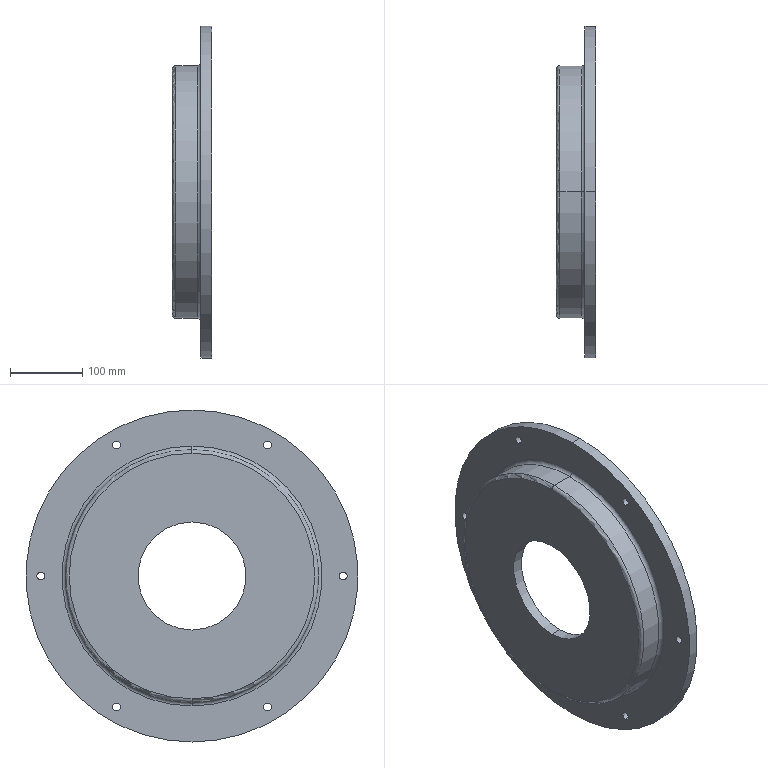Part | SolidWorks | features Cut 1, Revolution 1 | 1 solid | 32 faces | box 54.8 x 461 x 461 mm | volume 2855101 mm3 | cylinder 20 | torus 8 | plane 4 | commonest cylinder face diameters 11 x12 150 x2 321 x2 351 x2 461 x2
STEP:
#1=CARTESIAN_POINT('',(-352.644,210.,5.5));
#2=VERTEX_POINT('',#1);
#3=CARTESIAN_POINT('',(-352.644,210.,-5.5));
#4=VERTEX_POINT('',#3);
#5=CARTESIAN_POINT('',(-352.644,210.,0.));
#6=DIRECTION('',(1.,0.,0.));
#7=DIRECTION('',(0.,0.,-1.));
#8=AXIS2_PLACEMENT_3D('',#5,#6,#7);
#9=CIRCLE('',#8,5.5);
#10=EDGE_CURVE('',#2,#4,#9,.T.);
#11=ORIENTED_EDGE('',*,*,#10,.T.);
#12=CARTESIAN_POINT('',(-367.644,210.,-5.5));
#13=VERTEX_POINT('',#12);
#14=CARTESIAN_POINT('',(-282.644,210.,-5.5));
#15=DIRECTION('',(-1.,0.,0.));
#16=VECTOR('',#15,1000.);
#17=LINE('',#14,#16);
#18=EDGE_CURVE('',#4,#13,#17,.T.);
#19=ORIENTED_EDGE('',*,*,#18,.T.);
#20=CARTESIAN_POINT('',(-367.644,210.,5.5));
#21=VERTEX_POINT('',#20);
#22=CARTESIAN_POINT('',(-367.644,210.,0.));
#23=DIRECTION('',(-1.,0.,0.));
#24=DIRECTION('',(0.,0.,1.));
#25=AXIS2_PLACEMENT_3D('',#22,#23,#24);
#26=CIRCLE('',#25,5.5);
#27=EDGE_CURVE('',#13,#21,#26,.T.);
#28=ORIENTED_EDGE('',*,*,#27,.T.);
#29=CARTESIAN_POINT('',(-282.644,210.,5.5));
#30=DIRECTION('',(-1.,0.,0.));
#31=VECTOR('',#30,1000.);
#32=LINE('',#29,#31);
#33=EDGE_CURVE('',#2,#21,#32,.T.);
#34=ORIENTED_EDGE('',*,*,#33,.F.);
#35=EDGE_LOOP('',(#11,#19,#28,#34));
#36=FACE_OUTER_BOUND('',#35,.T.);
#37=CARTESIAN_POINT('',(-282.644,210.,0.));
#38=DIRECTION('',(-1.,0.,0.));
#39=DIRECTION('',(0.,0.,1.));
#40=AXIS2_PLACEMENT_3D('',#37,#38,#39);
#41=CYLINDRICAL_SURFACE('',#40,5.5);
#42=ADVANCED_FACE('',(#36),#41,.F.);
#43=CARTESIAN_POINT('',(-352.644,105.,-176.365));
#44=VERTEX_POINT('',#43);
#45=CARTESIAN_POINT('',(-352.644,105.,-187.365));
#46=VERTEX_POINT('',#45);
#47=CARTESIAN_POINT('',(-352.644,105.,-181.865));
#48=DIRECTION('',(1.,0.,0.));
#49=DIRECTION('',(0.,0.,-1.));
#50=AXIS2_PLACEMENT_3D('',#47,#48,#49);
#51=CIRCLE('',#50,5.5);
#52=EDGE_CURVE('',#44,#46,#51,.T.);
#53=ORIENTED_EDGE('',*,*,#52,.T.);
#54=CARTESIAN_POINT('',(-367.644,105.,-187.365));
#55=VERTEX_POINT('',#54);
#56=CARTESIAN_POINT('',(-282.644,105.,-187.365));
#57=DIRECTION('',(-1.,0.,0.));
#58=VECTOR('',#57,1000.);
#59=LINE('',#56,#58);
#60=EDGE_CURVE('',#46,#55,#59,.T.);
#61=ORIENTED_EDGE('',*,*,#60,.T.);
#62=CARTESIAN_POINT('',(-367.644,105.,-176.365));
#63=VERTEX_POINT('',#62);
#64=CARTESIAN_POINT('',(-367.644,105.,-181.865));
#65=DIRECTION('',(-1.,0.,0.));
#66=DIRECTION('',(0.,0.,1.));
#67=AXIS2_PLACEMENT_3D('',#64,#65,#66);
#68=CIRCLE('',#67,5.5);
#69=EDGE_CURVE('',#55,#63,#68,.T.);
#70=ORIENTED_EDGE('',*,*,#69,.T.);
#71=CARTESIAN_POINT('',(-282.644,105.,-176.365));
#72=DIRECTION('',(-1.,0.,0.));
#73=VECTOR('',#72,1000.);
#74=LINE('',#71,#73);
#75=EDGE_CURVE('',#44,#63,#74,.T.);
#76=ORIENTED_EDGE('',*,*,#75,.F.);
#77=EDGE_LOOP('',(#53,#61,#70,#76));
#78=FACE_OUTER_BOUND('',#77,.T.);
#79=CARTESIAN_POINT('',(-282.644,105.,-181.865));
#80=DIRECTION('',(-1.,0.,0.));
#81=DIRECTION('',(0.,0.,1.));
#82=AXIS2_PLACEMENT_3D('',#79,#80,#81);
#83=CYLINDRICAL_SURFACE('',#82,5.5);
#84=ADVANCED_FACE('',(#78),#83,.F.);
#85=CARTESIAN_POINT('',(-352.644,-105.,-176.365));
#86=VERTEX_POINT('',#85);
#87=CARTESIAN_POINT('',(-352.644,-105.,-187.365));
#88=VERTEX_POINT('',#87);
#89=CARTESIAN_POINT('',(-352.644,-105.,-181.865));
#90=DIRECTION('',(1.,0.,0.));
#91=DIRECTION('',(0.,0.,-1.));
#92=AXIS2_PLACEMENT_3D('',#89,#90,#91);
#93=CIRCLE('',#92,5.5);
#94=EDGE_CURVE('',#86,#88,#93,.T.);
#95=ORIENTED_EDGE('',*,*,#94,.T.);
#96=CARTESIAN_POINT('',(-367.644,-105.,-187.365));
#97=VERTEX_POINT('',#96);
#98=CARTESIAN_POINT('',(-282.644,-105.,-187.365));
#99=DIRECTION('',(-1.,0.,0.));
#100=VECTOR('',#99,1000.);
#101=LINE('',#98,#100);
#102=EDGE_CURVE('',#88,#97,#101,.T.);
#103=ORIENTED_EDGE('',*,*,#102,.T.);
#104=CARTESIAN_POINT('',(-367.644,-105.,-176.365));
#105=VERTEX_POINT('',#104);
#106=CARTESIAN_POINT('',(-367.644,-105.,-181.865));
#107=DIRECTION('',(-1.,0.,0.));
#108=DIRECTION('',(0.,0.,1.));
#109=AXIS2_PLACEMENT_3D('',#106,#107,#108);
#110=CIRCLE('',#109,5.5);
#111=EDGE_CURVE('',#97,#105,#110,.T.);
#112=ORIENTED_EDGE('',*,*,#111,.T.);
#113=CARTESIAN_POINT('',(-282.644,-105.,-176.365));
#114=DIRECTION('',(-1.,0.,0.));
#115=VECTOR('',#114,1000.);
#116=LINE('',#113,#115);
#117=EDGE_CURVE('',#86,#105,#116,.T.);
#118=ORIENTED_EDGE('',*,*,#117,.F.);
#119=EDGE_LOOP('',(#95,#103,#112,#118));
#120=FACE_OUTER_BOUND('',#119,.T.);
#121=CARTESIAN_POINT('',(-282.644,-105.,-181.865));
#122=DIRECTION('',(-1.,0.,0.));
#123=DIRECTION('',(0.,0.,1.));
#124=AXIS2_PLACEMENT_3D('',#121,#122,#123);
#125=CYLINDRICAL_SURFACE('',#124,5.5);
#126=ADVANCED_FACE('',(#120),#125,.F.);
#127=CARTESIAN_POINT('',(-352.644,-210.,5.5));
#128=VERTEX_POINT('',#127);
#129=CARTESIAN_POINT('',(-352.644,-210.,-5.5));
#130=VERTEX_POINT('',#129);
#131=CARTESIAN_POINT('',(-352.644,-210.,0.));
#132=DIRECTION('',(1.,0.,0.));
#133=DIRECTION('',(0.,0.,-1.));
#134=AXIS2_PLACEMENT_3D('',#131,#132,#133);
#135=CIRCLE('',#134,5.5);
#136=EDGE_CURVE('',#128,#130,#135,.T.);
#137=ORIENTED_EDGE('',*,*,#136,.T.);
#138=CARTESIAN_POINT('',(-367.644,-210.,-5.5));
#139=VERTEX_POINT('',#138);
#140=CARTESIAN_POINT('',(-282.644,-210.,-5.5));
#141=DIRECTION('',(-1.,0.,0.));
#142=VECTOR('',#141,1000.);
#143=LINE('',#140,#142);
#144=EDGE_CURVE('',#130,#139,#143,.T.);
#145=ORIENTED_EDGE('',*,*,#144,.T.);
#146=CARTESIAN_POINT('',(-367.644,-210.,5.5));
#147=VERTEX_POINT('',#146);
#148=CARTESIAN_POINT('',(-367.644,-210.,0.));
#149=DIRECTION('',(-1.,0.,0.));
#150=DIRECTION('',(0.,0.,1.));
#151=AXIS2_PLACEMENT_3D('',#148,#149,#150);
#152=CIRCLE('',#151,5.5);
#153=EDGE_CURVE('',#139,#147,#152,.T.);
#154=ORIENTED_EDGE('',*,*,#153,.T.);
#155=CARTESIAN_POINT('',(-282.644,-210.,5.5));
#156=DIRECTION('',(-1.,0.,0.));
#157=VECTOR('',#156,1000.);
#158=LINE('',#155,#157);
#159=EDGE_CURVE('',#128,#147,#158,.T.);
#160=ORIENTED_EDGE('',*,*,#159,.F.);
#161=EDGE_LOOP('',(#137,#145,#154,#160));
#162=FACE_OUTER_BOUND('',#161,.T.);
#163=CARTESIAN_POINT('',(-282.644,-210.,0.));
#164=DIRECTION('',(-1.,0.,0.));
#165=DIRECTION('',(0.,0.,1.));
#166=AXIS2_PLACEMENT_3D('',#163,#164,#165);
#167=CYLINDRICAL_SURFACE('',#166,5.5);
#168=ADVANCED_FACE('',(#162),#167,.F.);
#169=CARTESIAN_POINT('',(-352.644,-105.,187.365));
#170=VERTEX_POINT('',#169);
#171=CARTESIAN_POINT('',(-352.644,-105.,176.365));
#172=VERTEX_POINT('',#171);
#173=CARTESIAN_POINT('',(-352.644,-105.,181.865));
#174=DIRECTION('',(1.,0.,0.));
#175=DIRECTION('',(0.,0.,-1.));
#176=AXIS2_PLACEMENT_3D('',#173,#174,#175);
#177=CIRCLE('',#176,5.5);
#178=EDGE_CURVE('',#170,#172,#177,.T.);
#179=ORIENTED_EDGE('',*,*,#178,.T.);
#180=CARTESIAN_POINT('',(-367.644,-105.,176.365));
#181=VERTEX_POINT('',#180);
#182=CARTESIAN_POINT('',(-282.644,-105.,176.365));
#183=DIRECTION('',(-1.,0.,0.));
#184=VECTOR('',#183,1000.);
#185=LINE('',#182,#184);
#186=EDGE_CURVE('',#172,#181,#185,.T.);
#187=ORIENTED_EDGE('',*,*,#186,.T.);
#188=CARTESIAN_POINT('',(-367.644,-105.,187.365));
#189=VERTEX_POINT('',#188);
#190=CARTESIAN_POINT('',(-367.644,-105.,181.865));
#191=DIRECTION('',(-1.,0.,0.));
#192=DIRECTION('',(0.,0.,1.));
#193=AXIS2_PLACEMENT_3D('',#190,#191,#192);
#194=CIRCLE('',#193,5.5);
#195=EDGE_CURVE('',#181,#189,#194,.T.);
#196=ORIENTED_EDGE('',*,*,#195,.T.);
#197=CARTESIAN_POINT('',(-282.644,-105.,187.365));
#198=DIRECTION('',(-1.,0.,0.));
#199=VECTOR('',#198,1000.);
#200=LINE('',#197,#199);
#201=EDGE_CURVE('',#170,#189,#200,.T.);
#202=ORIENTED_EDGE('',*,*,#201,.F.);
#203=EDGE_LOOP('',(#179,#187,#196,#202));
#204=FACE_OUTER_BOUND('',#203,.T.);
#205=CARTESIAN_POINT('',(-282.644,-105.,181.865));
#206=DIRECTION('',(-1.,0.,0.));
#207=DIRECTION('',(0.,0.,1.));
#208=AXIS2_PLACEMENT_3D('',#205,#206,#207);
#209=CYLINDRICAL_SURFACE('',#208,5.5);
#210=ADVANCED_FACE('',(#204),#209,.F.);
#211=CARTESIAN_POINT('',(-352.644,105.,187.365));
#212=VERTEX_POINT('',#211);
#213=CARTESIAN_POINT('',(-352.644,105.,176.365));
#214=VERTEX_POINT('',#213);
#215=CARTESIAN_POINT('',(-352.644,105.,181.865));
#216=DIRECTION('',(1.,0.,0.));
#217=DIRECTION('',(0.,0.,-1.));
#218=AXIS2_PLACEMENT_3D('',#215,#216,#217);
#219=CIRCLE('',#218,5.5);
#220=EDGE_CURVE('',#212,#214,#219,.T.);
#221=ORIENTED_EDGE('',*,*,#220,.T.);
#222=CARTESIAN_POINT('',(-367.644,105.,176.365));
#223=VERTEX_POINT('',#222);
#224=CARTESIAN_POINT('',(-282.644,105.,176.365));
#225=DIRECTION('',(-1.,0.,0.));
#226=VECTOR('',#225,1000.);
#227=LINE('',#224,#226);
#228=EDGE_CURVE('',#214,#223,#227,.T.);
#229=ORIENTED_EDGE('',*,*,#228,.T.);
#230=CARTESIAN_POINT('',(-367.644,105.,187.365));
#231=VERTEX_POINT('',#230);
#232=CARTESIAN_POINT('',(-367.644,105.,181.865));
#233=DIRECTION('',(-1.,0.,0.));
#234=DIRECTION('',(0.,0.,1.));
#235=AXIS2_PLACEMENT_3D('',#232,#233,#234);
#236=CIRCLE('',#235,5.5);
#237=EDGE_CURVE('',#223,#231,#236,.T.);
#238=ORIENTED_EDGE('',*,*,#237,.T.);
#239=CARTESIAN_POINT('',(-282.644,105.,187.365));
#240=DIRECTION('',(-1.,0.,0.));
#241=VECTOR('',#240,1000.);
#242=LINE('',#239,#241);
#243=EDGE_CURVE('',#212,#231,#242,.T.);
#244=ORIENTED_EDGE('',*,*,#243,.F.);
#245=EDGE_LOOP('',(#221,#229,#238,#244));
#246=FACE_OUTER_BOUND('',#245,.T.);
#247=CARTESIAN_POINT('',(-282.644,105.,181.865));
#248=DIRECTION('',(-1.,0.,0.));
#249=DIRECTION('',(0.,0.,1.));
#250=AXIS2_PLACEMENT_3D('',#247,#248,#249);
#251=CYLINDRICAL_SURFACE('',#250,5.5);
#252=ADVANCED_FACE('',(#246),#251,.F.);
#253=CARTESIAN_POINT('',(-391.444,0.,160.5));
#254=VERTEX_POINT('',#253);
#255=CARTESIAN_POINT('',(-391.444,0.,-160.5));
#256=VERTEX_POINT('',#255);
#257=CARTESIAN_POINT('',(-391.444,0.,0.));
#258=DIRECTION('',(1.,0.,0.));
#259=DIRECTION('',(0.,0.,-1.));
#260=AXIS2_PLACEMENT_3D('',#257,#258,#259);
#261=CIRCLE('',#260,160.5);
#262=EDGE_CURVE('',#254,#256,#261,.T.);
#263=ORIENTED_EDGE('',*,*,#262,.F.);
#264=CARTESIAN_POINT('',(-357.644,0.,160.5));
#265=VERTEX_POINT('',#264);
#266=CARTESIAN_POINT('',(0.,0.,160.5));
#267=DIRECTION('',(1.,0.,0.));
#268=VECTOR('',#267,1000.);
#269=LINE('',#266,#268);
#270=EDGE_CURVE('',#254,#265,#269,.T.);
#271=ORIENTED_EDGE('',*,*,#270,.T.);
#272=CARTESIAN_POINT('',(-357.644,0.,-160.5));
#273=VERTEX_POINT('',#272);
#274=CARTESIAN_POINT('',(-357.644,0.,0.));
#275=DIRECTION('',(1.,0.,0.));
#276=DIRECTION('',(0.,0.,-1.));
#277=AXIS2_PLACEMENT_3D('',#274,#275,#276);
#278=CIRCLE('',#277,160.5);
#279=EDGE_CURVE('',#265,#273,#278,.T.);
#280=ORIENTED_EDGE('',*,*,#279,.T.);
#281=CARTESIAN_POINT('',(0.,0.,-160.5));
#282=DIRECTION('',(1.,0.,0.));
#283=VECTOR('',#282,1000.);
#284=LINE('',#281,#283);
#285=EDGE_CURVE('',#256,#273,#284,.T.);
#286=ORIENTED_EDGE('',*,*,#285,.F.);
#287=EDGE_LOOP('',(#263,#271,#280,#286));
#288=FACE_OUTER_BOUND('',#287,.T.);
#289=CARTESIAN_POINT('',(0.,0.,0.));
#290=DIRECTION('',(1.,0.,0.));
#291=DIRECTION('',(0.,0.,-1.));
#292=AXIS2_PLACEMENT_3D('',#289,#290,#291);
#293=CYLINDRICAL_SURFACE('',#292,160.5);
#294=ADVANCED_FACE('',(#288),#293,.F.);
#295=CARTESIAN_POINT('',(-392.444,0.,159.5));
#296=VERTEX_POINT('',#295);
#297=CARTESIAN_POINT('',(-392.444,0.,-159.5));
#298=VERTEX_POINT('',#297);
#299=CARTESIAN_POINT('',(-392.444,0.,0.));
#300=DIRECTION('',(1.,0.,0.));
#301=DIRECTION('',(0.,0.,-1.));
#302=AXIS2_PLACEMENT_3D('',#299,#300,#301);
#303=CIRCLE('',#302,159.5);
#304=EDGE_CURVE('',#296,#298,#303,.T.);
#305=ORIENTED_EDGE('',*,*,#304,.F.);
#306=CARTESIAN_POINT('',(-391.444,0.,159.5));
#307=DIRECTION('',(0.,1.,0.));
#308=DIRECTION('',(0.,0.,1.));
#309=AXIS2_PLACEMENT_3D('',#306,#307,#308);
#310=CIRCLE('',#309,1.);
#311=EDGE_CURVE('',#296,#254,#310,.T.);
#312=ORIENTED_EDGE('',*,*,#311,.T.);
#313=ORIENTED_EDGE('',*,*,#262,.T.);
#314=CARTESIAN_POINT('',(-391.444,0.,-159.5));
#315=DIRECTION('',(0.,-1.,0.));
#316=DIRECTION('',(0.,0.,-1.));
#317=AXIS2_PLACEMENT_3D('',#314,#315,#316);
#318=CIRCLE('',#317,1.);
#319=EDGE_CURVE('',#298,#256,#318,.T.);
#320=ORIENTED_EDGE('',*,*,#319,.F.);
#321=EDGE_LOOP('',(#305,#312,#313,#320));
#322=FACE_OUTER_BOUND('',#321,.T.);
#323=CARTESIAN_POINT('',(-391.444,0.,0.));
#324=DIRECTION('',(1.,0.,0.));
#325=DIRECTION('',(0.,0.,-1.));
#326=AXIS2_PLACEMENT_3D('',#323,#324,#325);
#327=TOROIDAL_SURFACE('',#326,159.5,1.);
#328=ADVANCED_FACE('',(#322),#327,.F.);
#329=CARTESIAN_POINT('',(-407.444,0.,75.));
#330=VERTEX_POINT('',#329);
#331=CARTESIAN_POINT('',(-407.444,0.,-75.));
#332=VERTEX_POINT('',#331);
#333=CARTESIAN_POINT('',(-407.444,0.,0.));
#334=DIRECTION('',(1.,0.,0.));
#335=DIRECTION('',(0.,0.,-1.));
#336=AXIS2_PLACEMENT_3D('',#333,#334,#335);
#337=CIRCLE('',#336,75.);
#338=EDGE_CURVE('',#330,#332,#337,.T.);
#339=ORIENTED_EDGE('',*,*,#338,.F.);
#340=CARTESIAN_POINT('',(-392.444,0.,75.));
#341=VERTEX_POINT('',#340);
#342=CARTESIAN_POINT('',(0.,0.,75.));
#343=DIRECTION('',(1.,0.,0.));
#344=VECTOR('',#343,1000.);
#345=LINE('',#342,#344);
#346=EDGE_CURVE('',#330,#341,#345,.T.);
#347=ORIENTED_EDGE('',*,*,#346,.T.);
#348=CARTESIAN_POINT('',(-392.444,0.,-75.));
#349=VERTEX_POINT('',#348);
#350=CARTESIAN_POINT('',(-392.444,0.,0.));
#351=DIRECTION('',(1.,0.,0.));
#352=DIRECTION('',(0.,0.,-1.));
#353=AXIS2_PLACEMENT_3D('',#350,#351,#352);
#354=CIRCLE('',#353,75.);
#355=EDGE_CURVE('',#341,#349,#354,.T.);
#356=ORIENTED_EDGE('',*,*,#355,.T.);
#357=CARTESIAN_POINT('',(0.,0.,-75.));
#358=DIRECTION('',(1.,0.,0.));
#359=VECTOR('',#358,1000.);
#360=LINE('',#357,#359);
#361=EDGE_CURVE('',#332,#349,#360,.T.);
#362=ORIENTED_EDGE('',*,*,#361,.F.);
#363=EDGE_LOOP('',(#339,#347,#356,#362));
#364=FACE_OUTER_BOUND('',#363,.T.);
#365=CARTESIAN_POINT('',(0.,0.,0.));
#366=DIRECTION('',(1.,0.,0.));
#367=DIRECTION('',(0.,0.,-1.));
#368=AXIS2_PLACEMENT_3D('',#365,#366,#367);
#369=CYLINDRICAL_SURFACE('',#368,75.);
#370=ADVANCED_FACE('',(#364),#369,.F.);
#371=CARTESIAN_POINT('',(-407.444,0.,-170.5));
#372=VERTEX_POINT('',#371);
#373=CARTESIAN_POINT('',(-407.444,0.,170.5));
#374=VERTEX_POINT('',#373);
#375=CARTESIAN_POINT('',(-407.444,0.,0.));
#376=DIRECTION('',(1.,0.,0.));
#377=DIRECTION('',(0.,0.,-1.));
#378=AXIS2_PLACEMENT_3D('',#375,#376,#377);
#379=CIRCLE('',#378,170.5);
#380=EDGE_CURVE('',#372,#374,#379,.T.);
#381=ORIENTED_EDGE('',*,*,#380,.T.);
#382=CARTESIAN_POINT('',(-402.444,0.,175.5));
#383=VERTEX_POINT('',#382);
#384=CARTESIAN_POINT('',(-402.444,0.,170.5));
#385=DIRECTION('',(0.,1.,0.));
#386=DIRECTION('',(0.,0.,1.));
#387=AXIS2_PLACEMENT_3D('',#384,#385,#386);
#388=CIRCLE('',#387,5.);
#389=EDGE_CURVE('',#374,#383,#388,.T.);
#390=ORIENTED_EDGE('',*,*,#389,.T.);
#391=CARTESIAN_POINT('',(-402.444,0.,-175.5));
#392=VERTEX_POINT('',#391);
#393=CARTESIAN_POINT('',(-402.444,0.,0.));
#394=DIRECTION('',(1.,0.,0.));
#395=DIRECTION('',(0.,0.,-1.));
#396=AXIS2_PLACEMENT_3D('',#393,#394,#395);
#397=CIRCLE('',#396,175.5);
#398=EDGE_CURVE('',#392,#383,#397,.T.);
#399=ORIENTED_EDGE('',*,*,#398,.F.);
#400=CARTESIAN_POINT('',(-402.444,0.,-170.5));
#401=DIRECTION('',(0.,-1.,0.));
#402=DIRECTION('',(0.,0.,-1.));
#403=AXIS2_PLACEMENT_3D('',#400,#401,#402);
#404=CIRCLE('',#403,5.);
#405=EDGE_CURVE('',#372,#392,#404,.T.);
#406=ORIENTED_EDGE('',*,*,#405,.F.);
#407=EDGE_LOOP('',(#381,#390,#399,#406));
#408=FACE_OUTER_BOUND('',#407,.T.);
#409=CARTESIAN_POINT('',(-402.444,0.,0.));
#410=DIRECTION('',(1.,0.,0.));
#411=DIRECTION('',(0.,0.,-1.));
#412=AXIS2_PLACEMENT_3D('',#409,#410,#411);
#413=TOROIDAL_SURFACE('',#412,170.5,5.);
#414=ADVANCED_FACE('',(#408),#413,.T.);
#415=ORIENTED_EDGE('',*,*,#398,.T.);
#416=CARTESIAN_POINT('',(-372.644,0.,175.5));
#417=VERTEX_POINT('',#416);
#418=CARTESIAN_POINT('',(0.,0.,175.5));
#419=DIRECTION('',(1.,0.,0.));
#420=VECTOR('',#419,1000.);
#421=LINE('',#418,#420);
#422=EDGE_CURVE('',#383,#417,#421,.T.);
#423=ORIENTED_EDGE('',*,*,#422,.T.);
#424=CARTESIAN_POINT('',(-372.644,0.,-175.5));
#425=VERTEX_POINT('',#424);
#426=CARTESIAN_POINT('',(-372.644,0.,0.));
#427=DIRECTION('',(1.,0.,0.));
#428=DIRECTION('',(0.,0.,-1.));
#429=AXIS2_PLACEMENT_3D('',#426,#427,#428);
#430=CIRCLE('',#429,175.5);
#431=EDGE_CURVE('',#425,#417,#430,.T.);
#432=ORIENTED_EDGE('',*,*,#431,.F.);
#433=CARTESIAN_POINT('',(0.,0.,-175.5));
#434=DIRECTION('',(1.,0.,0.));
#435=VECTOR('',#434,1000.);
#436=LINE('',#433,#435);
#437=EDGE_CURVE('',#392,#425,#436,.T.);
#438=ORIENTED_EDGE('',*,*,#437,.F.);
#439=EDGE_LOOP('',(#415,#423,#432,#438));
#440=FACE_OUTER_BOUND('',#439,.T.);
#441=CARTESIAN_POINT('',(0.,0.,0.));
#442=DIRECTION('',(1.,0.,0.));
#443=DIRECTION('',(0.,0.,-1.));
#444=AXIS2_PLACEMENT_3D('',#441,#442,#443);
#445=CYLINDRICAL_SURFACE('',#444,175.5);
#446=ADVANCED_FACE('',(#440),#445,.T.);
#447=CARTESIAN_POINT('',(-367.644,0.,180.5));
#448=VERTEX_POINT('',#447);
#449=CARTESIAN_POINT('',(-367.644,0.,-180.5));
#450=VERTEX_POINT('',#449);
#451=CARTESIAN_POINT('',(-367.644,0.,0.));
#452=DIRECTION('',(1.,0.,0.));
#453=DIRECTION('',(0.,0.,-1.));
#454=AXIS2_PLACEMENT_3D('',#451,#452,#453);
#455=CIRCLE('',#454,180.5);
#456=EDGE_CURVE('',#448,#450,#455,.T.);
#457=ORIENTED_EDGE('',*,*,#456,.F.);
#458=CARTESIAN_POINT('',(-372.644,0.,180.5));
#459=DIRECTION('',(0.,1.,0.));
#460=DIRECTION('',(0.,0.,1.));
#461=AXIS2_PLACEMENT_3D('',#458,#459,#460);
#462=CIRCLE('',#461,5.);
#463=EDGE_CURVE('',#448,#417,#462,.T.);
#464=ORIENTED_EDGE('',*,*,#463,.T.);
#465=CARTESIAN_POINT('',(-372.644,0.,0.));
#466=DIRECTION('',(1.,0.,0.));
#467=DIRECTION('',(0.,0.,-1.));
#468=AXIS2_PLACEMENT_3D('',#465,#466,#467);
#469=CIRCLE('',#468,175.5);
#470=EDGE_CURVE('',#417,#425,#469,.T.);
#471=ORIENTED_EDGE('',*,*,#470,.T.);
#472=CARTESIAN_POINT('',(-372.644,0.,-180.5));
#473=DIRECTION('',(0.,-1.,0.));
#474=DIRECTION('',(0.,0.,-1.));
#475=AXIS2_PLACEMENT_3D('',#472,#473,#474);
#476=CIRCLE('',#475,5.);
#477=EDGE_CURVE('',#450,#425,#476,.T.);
#478=ORIENTED_EDGE('',*,*,#477,.F.);
#479=EDGE_LOOP('',(#457,#464,#471,#478));
#480=FACE_OUTER_BOUND('',#479,.T.);
#481=CARTESIAN_POINT('',(-372.644,0.,0.));
#482=DIRECTION('',(1.,0.,0.));
#483=DIRECTION('',(0.,0.,-1.));
#484=AXIS2_PLACEMENT_3D('',#481,#482,#483);
#485=TOROIDAL_SURFACE('',#484,180.5,5.);
#486=ADVANCED_FACE('',(#480),#485,.F.);
#487=CARTESIAN_POINT('',(-367.644,0.,-230.5));
#488=VERTEX_POINT('',#487);
#489=CARTESIAN_POINT('',(-367.644,0.,230.5));
#490=VERTEX_POINT('',#489);
#491=CARTESIAN_POINT('',(-367.644,0.,0.));
#492=DIRECTION('',(1.,0.,0.));
#493=DIRECTION('',(0.,0.,-1.));
#494=AXIS2_PLACEMENT_3D('',#491,#492,#493);
#495=CIRCLE('',#494,230.5);
#496=EDGE_CURVE('',#488,#490,#495,.T.);
#497=ORIENTED_EDGE('',*,*,#496,.T.);
#498=CARTESIAN_POINT('',(-352.644,0.,230.5));
#499=VERTEX_POINT('',#498);
#500=CARTESIAN_POINT('',(0.,0.,230.5));
#501=DIRECTION('',(1.,0.,0.));
#502=VECTOR('',#501,1000.);
#503=LINE('',#500,#502);
#504=EDGE_CURVE('',#490,#499,#503,.T.);
#505=ORIENTED_EDGE('',*,*,#504,.T.);
#506=CARTESIAN_POINT('',(-352.644,0.,-230.5));
#507=VERTEX_POINT('',#506);
#508=CARTESIAN_POINT('',(-352.644,0.,0.));
#509=DIRECTION('',(1.,0.,0.));
#510=DIRECTION('',(0.,0.,-1.));
#511=AXIS2_PLACEMENT_3D('',#508,#509,#510);
#512=CIRCLE('',#511,230.5);
#513=EDGE_CURVE('',#507,#499,#512,.T.);
#514=ORIENTED_EDGE('',*,*,#513,.F.);
#515=CARTESIAN_POINT('',(0.,0.,-230.5));
#516=DIRECTION('',(1.,0.,0.));
#517=VECTOR('',#516,1000.);
#518=LINE('',#515,#517);
#519=EDGE_CURVE('',#488,#507,#518,.T.);
#520=ORIENTED_EDGE('',*,*,#519,.F.);
#521=EDGE_LOOP('',(#497,#505,#514,#520));
#522=FACE_OUTER_BOUND('',#521,.T.);
#523=CARTESIAN_POINT('',(0.,0.,0.));
#524=DIRECTION('',(1.,0.,0.));
#525=DIRECTION('',(0.,0.,-1.));
#526=AXIS2_PLACEMENT_3D('',#523,#524,#525);
#527=CYLINDRICAL_SURFACE('',#526,230.5);
#528=ADVANCED_FACE('',(#522),#527,.T.);
#529=CARTESIAN_POINT('',(-352.644,0.,-165.5));
#530=VERTEX_POINT('',#529);
#531=CARTESIAN_POINT('',(-352.644,0.,165.5));
#532=VERTEX_POINT('',#531);
#533=CARTESIAN_POINT('',(-352.644,0.,0.));
#534=DIRECTION('',(1.,0.,0.));
#535=DIRECTION('',(0.,0.,-1.));
#536=AXIS2_PLACEMENT_3D('',#533,#534,#535);
#537=CIRCLE('',#536,165.5);
#538=EDGE_CURVE('',#530,#532,#537,.T.);
#539=ORIENTED_EDGE('',*,*,#538,.T.);
#540=CARTESIAN_POINT('',(-357.644,0.,165.5));
#541=DIRECTION('',(0.,1.,0.));
#542=DIRECTION('',(0.,0.,1.));
#543=AXIS2_PLACEMENT_3D('',#540,#541,#542);
#544=CIRCLE('',#543,5.);
#545=EDGE_CURVE('',#532,#265,#544,.T.);
#546=ORIENTED_EDGE('',*,*,#545,.T.);
#547=CARTESIAN_POINT('',(-357.644,0.,0.));
#548=DIRECTION('',(1.,0.,0.));
#549=DIRECTION('',(0.,0.,-1.));
#550=AXIS2_PLACEMENT_3D('',#547,#548,#549);
#551=CIRCLE('',#550,160.5);
#552=EDGE_CURVE('',#273,#265,#551,.T.);
#553=ORIENTED_EDGE('',*,*,#552,.F.);
#554=CARTESIAN_POINT('',(-357.644,0.,-165.5));
#555=DIRECTION('',(0.,-1.,0.));
#556=DIRECTION('',(0.,0.,-1.));
#557=AXIS2_PLACEMENT_3D('',#554,#555,#556);
#558=CIRCLE('',#557,5.);
#559=EDGE_CURVE('',#530,#273,#558,.T.);
#560=ORIENTED_EDGE('',*,*,#559,.F.);
#561=EDGE_LOOP('',(#539,#546,#553,#560));
#562=FACE_OUTER_BOUND('',#561,.T.);
#563=CARTESIAN_POINT('',(-357.644,0.,0.));
#564=DIRECTION('',(1.,0.,0.));
#565=DIRECTION('',(0.,0.,-1.));
#566=AXIS2_PLACEMENT_3D('',#563,#564,#565);
#567=TOROIDAL_SURFACE('',#566,165.5,5.);
#568=ADVANCED_FACE('',(#562),#567,.T.);
#569=ORIENTED_EDGE('',*,*,#545,.F.);
#570=CARTESIAN_POINT('',(-352.644,0.,0.));
#571=DIRECTION('',(1.,0.,0.));
#572=DIRECTION('',(0.,0.,-1.));
#573=AXIS2_PLACEMENT_3D('',#570,#571,#572);
#574=CIRCLE('',#573,165.5);
#575=EDGE_CURVE('',#532,#530,#574,.T.);
#576=ORIENTED_EDGE('',*,*,#575,.T.);
#577=ORIENTED_EDGE('',*,*,#559,.T.);
#578=ORIENTED_EDGE('',*,*,#279,.F.);
#579=EDGE_LOOP('',(#569,#576,#577,#578));
#580=FACE_OUTER_BOUND('',#579,.T.);
#581=CARTESIAN_POINT('',(-357.644,0.,0.));
#582=DIRECTION('',(1.,0.,0.));
#583=DIRECTION('',(0.,0.,-1.));
#584=AXIS2_PLACEMENT_3D('',#581,#582,#583);
#585=TOROIDAL_SURFACE('',#584,165.5,5.);
#586=ADVANCED_FACE('',(#580),#585,.T.);
#587=ORIENTED_EDGE('',*,*,#10,.F.);
#588=CARTESIAN_POINT('',(-352.644,210.,0.));
#589=DIRECTION('',(1.,0.,0.));
#590=DIRECTION('',(0.,0.,-1.));
#591=AXIS2_PLACEMENT_3D('',#588,#589,#590);
#592=CIRCLE('',#591,5.5);
#593=EDGE_CURVE('',#4,#2,#592,.T.);
#594=ORIENTED_EDGE('',*,*,#593,.F.);
#595=EDGE_LOOP('',(#587,#594));
#596=FACE_BOUND('',#595,.T.);
#597=ORIENTED_EDGE('',*,*,#52,.F.);
#598=CARTESIAN_POINT('',(-352.644,105.,-181.865));
#599=DIRECTION('',(1.,0.,0.));
#600=DIRECTION('',(0.,0.,-1.));
#601=AXIS2_PLACEMENT_3D('',#598,#599,#600);
#602=CIRCLE('',#601,5.5);
#603=EDGE_CURVE('',#46,#44,#602,.T.);
#604=ORIENTED_EDGE('',*,*,#603,.F.);
#605=EDGE_LOOP('',(#597,#604));
#606=FACE_BOUND('',#605,.T.);
#607=ORIENTED_EDGE('',*,*,#94,.F.);
#608=CARTESIAN_POINT('',(-352.644,-105.,-181.865));
#609=DIRECTION('',(1.,0.,0.));
#610=DIRECTION('',(0.,0.,-1.));
#611=AXIS2_PLACEMENT_3D('',#608,#609,#610);
#612=CIRCLE('',#611,5.5);
#613=EDGE_CURVE('',#88,#86,#612,.T.);
#614=ORIENTED_EDGE('',*,*,#613,.F.);
#615=EDGE_LOOP('',(#607,#614));
#616=FACE_BOUND('',#615,.T.);
#617=ORIENTED_EDGE('',*,*,#136,.F.);
#618=CARTESIAN_POINT('',(-352.644,-210.,0.));
#619=DIRECTION('',(1.,0.,0.));
#620=DIRECTION('',(0.,0.,-1.));
#621=AXIS2_PLACEMENT_3D('',#618,#619,#620);
#622=CIRCLE('',#621,5.5);
#623=EDGE_CURVE('',#130,#128,#622,.T.);
#624=ORIENTED_EDGE('',*,*,#623,.F.);
#625=EDGE_LOOP('',(#617,#624));
#626=FACE_BOUND('',#625,.T.);
#627=ORIENTED_EDGE('',*,*,#178,.F.);
#628=CARTESIAN_POINT('',(-352.644,-105.,181.865));
#629=DIRECTION('',(1.,0.,0.));
#630=DIRECTION('',(0.,0.,-1.));
#631=AXIS2_PLACEMENT_3D('',#628,#629,#630);
#632=CIRCLE('',#631,5.5);
#633=EDGE_CURVE('',#172,#170,#632,.T.);
#634=ORIENTED_EDGE('',*,*,#633,.F.);
#635=EDGE_LOOP('',(#627,#634));
#636=FACE_BOUND('',#635,.T.);
#637=ORIENTED_EDGE('',*,*,#220,.F.);
#638=CARTESIAN_POINT('',(-352.644,105.,181.865));
#639=DIRECTION('',(1.,0.,0.));
#640=DIRECTION('',(0.,0.,-1.));
#641=AXIS2_PLACEMENT_3D('',#638,#639,#640);
#642=CIRCLE('',#641,5.5);
#643=EDGE_CURVE('',#214,#212,#642,.T.);
#644=ORIENTED_EDGE('',*,*,#643,.F.);
#645=EDGE_LOOP('',(#637,#644));
#646=FACE_BOUND('',#645,.T.);
#647=ORIENTED_EDGE('',*,*,#513,.T.);
#648=CARTESIAN_POINT('',(-352.644,0.,0.));
#649=DIRECTION('',(1.,0.,0.));
#650=DIRECTION('',(0.,0.,-1.));
#651=AXIS2_PLACEMENT_3D('',#648,#649,#650);
#652=CIRCLE('',#651,230.5);
#653=EDGE_CURVE('',#499,#507,#652,.T.);
#654=ORIENTED_EDGE('',*,*,#653,.T.);
#655=EDGE_LOOP('',(#647,#654));
#656=FACE_OUTER_BOUND('',#655,.T.);
#657=ORIENTED_EDGE('',*,*,#538,.F.);
#658=ORIENTED_EDGE('',*,*,#575,.F.);
#659=EDGE_LOOP('',(#657,#658));
#660=FACE_BOUND('',#659,.T.);
#661=CARTESIAN_POINT('',(-352.644,230.5,0.));
#662=DIRECTION('',(1.,0.,0.));
#663=DIRECTION('',(0.,0.,-1.));
#664=AXIS2_PLACEMENT_3D('',#661,#662,#663);
#665=PLANE('',#664);
#666=ADVANCED_FACE('',(#596,#606,#616,#626,#636,#646,#656,#660),#665,.T.);
#667=ORIENTED_EDGE('',*,*,#504,.F.);
#668=CARTESIAN_POINT('',(-367.644,0.,0.));
#669=DIRECTION('',(1.,0.,0.));
#670=DIRECTION('',(0.,0.,-1.));
#671=AXIS2_PLACEMENT_3D('',#668,#669,#670);
#672=CIRCLE('',#671,230.5);
#673=EDGE_CURVE('',#490,#488,#672,.T.);
#674=ORIENTED_EDGE('',*,*,#673,.T.);
#675=ORIENTED_EDGE('',*,*,#519,.T.);
#676=ORIENTED_EDGE('',*,*,#653,.F.);
#677=EDGE_LOOP('',(#667,#674,#675,#676));
#678=FACE_OUTER_BOUND('',#677,.T.);
#679=CARTESIAN_POINT('',(0.,0.,0.));
#680=DIRECTION('',(1.,0.,0.));
#681=DIRECTION('',(0.,0.,-1.));
#682=AXIS2_PLACEMENT_3D('',#679,#680,#681);
#683=CYLINDRICAL_SURFACE('',#682,230.5);
#684=ADVANCED_FACE('',(#678),#683,.T.);
#685=CARTESIAN_POINT('',(-367.644,210.,0.));
#686=DIRECTION('',(-1.,0.,0.));
#687=DIRECTION('',(0.,0.,1.));
#688=AXIS2_PLACEMENT_3D('',#685,#686,#687);
#689=CIRCLE('',#688,5.5);
#690=EDGE_CURVE('',#21,#13,#689,.T.);
#691=ORIENTED_EDGE('',*,*,#690,.F.);
#692=ORIENTED_EDGE('',*,*,#27,.F.);
#693=EDGE_LOOP('',(#691,#692));
#694=FACE_BOUND('',#693,.T.);
#695=CARTESIAN_POINT('',(-367.644,105.,-181.865));
#696=DIRECTION('',(-1.,0.,0.));
#697=DIRECTION('',(0.,0.,1.));
#698=AXIS2_PLACEMENT_3D('',#695,#696,#697);
#699=CIRCLE('',#698,5.5);
#700=EDGE_CURVE('',#63,#55,#699,.T.);
#701=ORIENTED_EDGE('',*,*,#700,.F.);
#702=ORIENTED_EDGE('',*,*,#69,.F.);
#703=EDGE_LOOP('',(#701,#702));
#704=FACE_BOUND('',#703,.T.);
#705=CARTESIAN_POINT('',(-367.644,-105.,-181.865));
#706=DIRECTION('',(-1.,0.,0.));
#707=DIRECTION('',(0.,0.,1.));
#708=AXIS2_PLACEMENT_3D('',#705,#706,#707);
#709=CIRCLE('',#708,5.5);
#710=EDGE_CURVE('',#105,#97,#709,.T.);
#711=ORIENTED_EDGE('',*,*,#710,.F.);
#712=ORIENTED_EDGE('',*,*,#111,.F.);
#713=EDGE_LOOP('',(#711,#712));
#714=FACE_BOUND('',#713,.T.);
#715=CARTESIAN_POINT('',(-367.644,-210.,0.));
#716=DIRECTION('',(-1.,0.,0.));
#717=DIRECTION('',(0.,0.,1.));
#718=AXIS2_PLACEMENT_3D('',#715,#716,#717);
#719=CIRCLE('',#718,5.5);
#720=EDGE_CURVE('',#147,#139,#719,.T.);
#721=ORIENTED_EDGE('',*,*,#720,.F.);
#722=ORIENTED_EDGE('',*,*,#153,.F.);
#723=EDGE_LOOP('',(#721,#722));
#724=FACE_BOUND('',#723,.T.);
#725=CARTESIAN_POINT('',(-367.644,-105.,181.865));
#726=DIRECTION('',(-1.,0.,0.));
#727=DIRECTION('',(0.,0.,1.));
#728=AXIS2_PLACEMENT_3D('',#725,#726,#727);
#729=CIRCLE('',#728,5.5);
#730=EDGE_CURVE('',#189,#181,#729,.T.);
#731=ORIENTED_EDGE('',*,*,#730,.F.);
#732=ORIENTED_EDGE('',*,*,#195,.F.);
#733=EDGE_LOOP('',(#731,#732));
#734=FACE_BOUND('',#733,.T.);
#735=CARTESIAN_POINT('',(-367.644,105.,181.865));
#736=DIRECTION('',(-1.,0.,0.));
#737=DIRECTION('',(0.,0.,1.));
#738=AXIS2_PLACEMENT_3D('',#735,#736,#737);
#739=CIRCLE('',#738,5.5);
#740=EDGE_CURVE('',#231,#223,#739,.T.);
#741=ORIENTED_EDGE('',*,*,#740,.F.);
#742=ORIENTED_EDGE('',*,*,#237,.F.);
#743=EDGE_LOOP('',(#741,#742));
#744=FACE_BOUND('',#743,.T.);
#745=CARTESIAN_POINT('',(-367.644,0.,0.));
#746=DIRECTION('',(1.,0.,0.));
#747=DIRECTION('',(0.,0.,-1.));
#748=AXIS2_PLACEMENT_3D('',#745,#746,#747);
#749=CIRCLE('',#748,180.5);
#750=EDGE_CURVE('',#450,#448,#749,.T.);
#751=ORIENTED_EDGE('',*,*,#750,.T.);
#752=ORIENTED_EDGE('',*,*,#456,.T.);
#753=EDGE_LOOP('',(#751,#752));
#754=FACE_BOUND('',#753,.T.);
#755=ORIENTED_EDGE('',*,*,#496,.F.);
#756=ORIENTED_EDGE('',*,*,#673,.F.);
#757=EDGE_LOOP('',(#755,#756));
#758=FACE_OUTER_BOUND('',#757,.T.);
#759=CARTESIAN_POINT('',(-367.644,205.,0.));
#760=DIRECTION('',(-1.,0.,0.));
#761=DIRECTION('',(0.,0.,1.));
#762=AXIS2_PLACEMENT_3D('',#759,#760,#761);
#763=PLANE('',#762);
#764=ADVANCED_FACE('',(#694,#704,#714,#724,#734,#744,#754,#758),#763,.T.);
#765=ORIENTED_EDGE('',*,*,#463,.F.);
#766=ORIENTED_EDGE('',*,*,#750,.F.);
#767=ORIENTED_EDGE('',*,*,#477,.T.);
#768=ORIENTED_EDGE('',*,*,#431,.T.);
#769=EDGE_LOOP('',(#765,#766,#767,#768));
#770=FACE_OUTER_BOUND('',#769,.T.);
#771=CARTESIAN_POINT('',(-372.644,0.,0.));
#772=DIRECTION('',(1.,0.,0.));
#773=DIRECTION('',(0.,0.,-1.));
#774=AXIS2_PLACEMENT_3D('',#771,#772,#773);
#775=TOROIDAL_SURFACE('',#774,180.5,5.);
#776=ADVANCED_FACE('',(#770),#775,.F.);
#777=ORIENTED_EDGE('',*,*,#422,.F.);
#778=CARTESIAN_POINT('',(-402.444,0.,0.));
#779=DIRECTION('',(1.,0.,0.));
#780=DIRECTION('',(0.,0.,-1.));
#781=AXIS2_PLACEMENT_3D('',#778,#779,#780);
#782=CIRCLE('',#781,175.5);
#783=EDGE_CURVE('',#383,#392,#782,.T.);
#784=ORIENTED_EDGE('',*,*,#783,.T.);
#785=ORIENTED_EDGE('',*,*,#437,.T.);
#786=ORIENTED_EDGE('',*,*,#470,.F.);
#787=EDGE_LOOP('',(#777,#784,#785,#786));
#788=FACE_OUTER_BOUND('',#787,.T.);
#789=CARTESIAN_POINT('',(0.,0.,0.));
#790=DIRECTION('',(1.,0.,0.));
#791=DIRECTION('',(0.,0.,-1.));
#792=AXIS2_PLACEMENT_3D('',#789,#790,#791);
#793=CYLINDRICAL_SURFACE('',#792,175.5);
#794=ADVANCED_FACE('',(#788),#793,.T.);
#795=ORIENTED_EDGE('',*,*,#389,.F.);
#796=CARTESIAN_POINT('',(-407.444,0.,0.));
#797=DIRECTION('',(1.,0.,0.));
#798=DIRECTION('',(0.,0.,-1.));
#799=AXIS2_PLACEMENT_3D('',#796,#797,#798);
#800=CIRCLE('',#799,170.5);
#801=EDGE_CURVE('',#374,#372,#800,.T.);
#802=ORIENTED_EDGE('',*,*,#801,.T.);
#803=ORIENTED_EDGE('',*,*,#405,.T.);
#804=ORIENTED_EDGE('',*,*,#783,.F.);
#805=EDGE_LOOP('',(#795,#802,#803,#804));
#806=FACE_OUTER_BOUND('',#805,.T.);
#807=CARTESIAN_POINT('',(-402.444,0.,0.));
#808=DIRECTION('',(1.,0.,0.));
#809=DIRECTION('',(0.,0.,-1.));
#810=AXIS2_PLACEMENT_3D('',#807,#808,#809);
#811=TOROIDAL_SURFACE('',#810,170.5,5.);
#812=ADVANCED_FACE('',(#806),#811,.T.);
#813=CARTESIAN_POINT('',(-407.444,0.,0.));
#814=DIRECTION('',(1.,0.,0.));
#815=DIRECTION('',(0.,0.,-1.));
#816=AXIS2_PLACEMENT_3D('',#813,#814,#815);
#817=CIRCLE('',#816,75.);
#818=EDGE_CURVE('',#332,#330,#817,.T.);
#819=ORIENTED_EDGE('',*,*,#818,.T.);
#820=ORIENTED_EDGE('',*,*,#338,.T.);
#821=EDGE_LOOP('',(#819,#820));
#822=FACE_BOUND('',#821,.T.);
#823=ORIENTED_EDGE('',*,*,#380,.F.);
#824=ORIENTED_EDGE('',*,*,#801,.F.);
#825=EDGE_LOOP('',(#823,#824));
#826=FACE_OUTER_BOUND('',#825,.T.);
#827=CARTESIAN_POINT('',(-407.444,131.,0.));
#828=DIRECTION('',(-1.,0.,0.));
#829=DIRECTION('',(0.,0.,1.));
#830=AXIS2_PLACEMENT_3D('',#827,#828,#829);
#831=PLANE('',#830);
#832=ADVANCED_FACE('',(#822,#826),#831,.T.);
#833=ORIENTED_EDGE('',*,*,#346,.F.);
#834=ORIENTED_EDGE('',*,*,#818,.F.);
#835=ORIENTED_EDGE('',*,*,#361,.T.);
#836=CARTESIAN_POINT('',(-392.444,0.,0.));
#837=DIRECTION('',(1.,0.,0.));
#838=DIRECTION('',(0.,0.,-1.));
#839=AXIS2_PLACEMENT_3D('',#836,#837,#838);
#840=CIRCLE('',#839,75.);
#841=EDGE_CURVE('',#349,#341,#840,.T.);
#842=ORIENTED_EDGE('',*,*,#841,.T.);
#843=EDGE_LOOP('',(#833,#834,#835,#842));
#844=FACE_OUTER_BOUND('',#843,.T.);
#845=CARTESIAN_POINT('',(0.,0.,0.));
#846=DIRECTION('',(1.,0.,0.));
#847=DIRECTION('',(0.,0.,-1.));
#848=AXIS2_PLACEMENT_3D('',#845,#846,#847);
#849=CYLINDRICAL_SURFACE('',#848,75.);
#850=ADVANCED_FACE('',(#844),#849,.F.);
#851=CARTESIAN_POINT('',(-392.444,0.,0.));
#852=DIRECTION('',(1.,0.,0.));
#853=DIRECTION('',(0.,0.,-1.));
#854=AXIS2_PLACEMENT_3D('',#851,#852,#853);
#855=CIRCLE('',#854,159.5);
#856=EDGE_CURVE('',#298,#296,#855,.T.);
#857=ORIENTED_EDGE('',*,*,#856,.T.);
#858=ORIENTED_EDGE('',*,*,#304,.T.);
#859=EDGE_LOOP('',(#857,#858));
#860=FACE_OUTER_BOUND('',#859,.T.);
#861=ORIENTED_EDGE('',*,*,#841,.F.);
#862=ORIENTED_EDGE('',*,*,#355,.F.);
#863=EDGE_LOOP('',(#861,#862));
#864=FACE_BOUND('',#863,.T.);
#865=CARTESIAN_POINT('',(-392.444,159.5,0.));
#866=DIRECTION('',(1.,0.,0.));
#867=DIRECTION('',(0.,0.,-1.));
#868=AXIS2_PLACEMENT_3D('',#865,#866,#867);
#869=PLANE('',#868);
#870=ADVANCED_FACE('',(#860,#864),#869,.T.);
#871=ORIENTED_EDGE('',*,*,#311,.F.);
#872=ORIENTED_EDGE('',*,*,#856,.F.);
#873=ORIENTED_EDGE('',*,*,#319,.T.);
#874=CARTESIAN_POINT('',(-391.444,0.,0.));
#875=DIRECTION('',(1.,0.,0.));
#876=DIRECTION('',(0.,0.,-1.));
#877=AXIS2_PLACEMENT_3D('',#874,#875,#876);
#878=CIRCLE('',#877,160.5);
#879=EDGE_CURVE('',#256,#254,#878,.T.);
#880=ORIENTED_EDGE('',*,*,#879,.T.);
#881=EDGE_LOOP('',(#871,#872,#873,#880));
#882=FACE_OUTER_BOUND('',#881,.T.);
#883=CARTESIAN_POINT('',(-391.444,0.,0.));
#884=DIRECTION('',(1.,0.,0.));
#885=DIRECTION('',(0.,0.,-1.));
#886=AXIS2_PLACEMENT_3D('',#883,#884,#885);
#887=TOROIDAL_SURFACE('',#886,159.5,1.);
#888=ADVANCED_FACE('',(#882),#887,.F.);
#889=ORIENTED_EDGE('',*,*,#270,.F.);
#890=ORIENTED_EDGE('',*,*,#879,.F.);
#891=ORIENTED_EDGE('',*,*,#285,.T.);
#892=ORIENTED_EDGE('',*,*,#552,.T.);
#893=EDGE_LOOP('',(#889,#890,#891,#892));
#894=FACE_OUTER_BOUND('',#893,.T.);
#895=CARTESIAN_POINT('',(0.,0.,0.));
#896=DIRECTION('',(1.,0.,0.));
#897=DIRECTION('',(0.,0.,-1.));
#898=AXIS2_PLACEMENT_3D('',#895,#896,#897);
#899=CYLINDRICAL_SURFACE('',#898,160.5);
#900=ADVANCED_FACE('',(#894),#899,.F.);
#901=ORIENTED_EDGE('',*,*,#228,.F.);
#902=ORIENTED_EDGE('',*,*,#643,.T.);
#903=ORIENTED_EDGE('',*,*,#243,.T.);
#904=ORIENTED_EDGE('',*,*,#740,.T.);
#905=EDGE_LOOP('',(#901,#902,#903,#904));
#906=FACE_OUTER_BOUND('',#905,.T.);
#907=CARTESIAN_POINT('',(-282.644,105.,181.865));
#908=DIRECTION('',(-1.,0.,0.));
#909=DIRECTION('',(0.,0.,1.));
#910=AXIS2_PLACEMENT_3D('',#907,#908,#909);
#911=CYLINDRICAL_SURFACE('',#910,5.5);
#912=ADVANCED_FACE('',(#906),#911,.F.);
#913=ORIENTED_EDGE('',*,*,#186,.F.);
#914=ORIENTED_EDGE('',*,*,#633,.T.);
#915=ORIENTED_EDGE('',*,*,#201,.T.);
#916=ORIENTED_EDGE('',*,*,#730,.T.);
#917=EDGE_LOOP('',(#913,#914,#915,#916));
#918=FACE_OUTER_BOUND('',#917,.T.);
#919=CARTESIAN_POINT('',(-282.644,-105.,181.865));
#920=DIRECTION('',(-1.,0.,0.));
#921=DIRECTION('',(0.,0.,1.));
#922=AXIS2_PLACEMENT_3D('',#919,#920,#921);
#923=CYLINDRICAL_SURFACE('',#922,5.5);
#924=ADVANCED_FACE('',(#918),#923,.F.);
#925=ORIENTED_EDGE('',*,*,#144,.F.);
#926=ORIENTED_EDGE('',*,*,#623,.T.);
#927=ORIENTED_EDGE('',*,*,#159,.T.);
#928=ORIENTED_EDGE('',*,*,#720,.T.);
#929=EDGE_LOOP('',(#925,#926,#927,#928));
#930=FACE_OUTER_BOUND('',#929,.T.);
#931=CARTESIAN_POINT('',(-282.644,-210.,0.));
#932=DIRECTION('',(-1.,0.,0.));
#933=DIRECTION('',(0.,0.,1.));
#934=AXIS2_PLACEMENT_3D('',#931,#932,#933);
#935=CYLINDRICAL_SURFACE('',#934,5.5);
#936=ADVANCED_FACE('',(#930),#935,.F.);
#937=ORIENTED_EDGE('',*,*,#102,.F.);
#938=ORIENTED_EDGE('',*,*,#613,.T.);
#939=ORIENTED_EDGE('',*,*,#117,.T.);
#940=ORIENTED_EDGE('',*,*,#710,.T.);
#941=EDGE_LOOP('',(#937,#938,#939,#940));
#942=FACE_OUTER_BOUND('',#941,.T.);
#943=CARTESIAN_POINT('',(-282.644,-105.,-181.865));
#944=DIRECTION('',(-1.,0.,0.));
#945=DIRECTION('',(0.,0.,1.));
#946=AXIS2_PLACEMENT_3D('',#943,#944,#945);
#947=CYLINDRICAL_SURFACE('',#946,5.5);
#948=ADVANCED_FACE('',(#942),#947,.F.);
#949=ORIENTED_EDGE('',*,*,#60,.F.);
#950=ORIENTED_EDGE('',*,*,#603,.T.);
#951=ORIENTED_EDGE('',*,*,#75,.T.);
#952=ORIENTED_EDGE('',*,*,#700,.T.);
#953=EDGE_LOOP('',(#949,#950,#951,#952));
#954=FACE_OUTER_BOUND('',#953,.T.);
#955=CARTESIAN_POINT('',(-282.644,105.,-181.865));
#956=DIRECTION('',(-1.,0.,0.));
#957=DIRECTION('',(0.,0.,1.));
#958=AXIS2_PLACEMENT_3D('',#955,#956,#957);
#959=CYLINDRICAL_SURFACE('',#958,5.5);
#960=ADVANCED_FACE('',(#954),#959,.F.);
#961=ORIENTED_EDGE('',*,*,#18,.F.);
#962=ORIENTED_EDGE('',*,*,#593,.T.);
#963=ORIENTED_EDGE('',*,*,#33,.T.);
#964=ORIENTED_EDGE('',*,*,#690,.T.);
#965=EDGE_LOOP('',(#961,#962,#963,#964));
#966=FACE_OUTER_BOUND('',#965,.T.);
#967=CARTESIAN_POINT('',(-282.644,210.,0.));
#968=DIRECTION('',(-1.,0.,0.));
#969=DIRECTION('',(0.,0.,1.));
#970=AXIS2_PLACEMENT_3D('',#967,#968,#969);
#971=CYLINDRICAL_SURFACE('',#970,5.5);
#972=ADVANCED_FACE('',(#966),#971,.F.);
#973=CLOSED_SHELL('',(#42,#84,#126,#168,#210,#252,#294,#328,#370,#414,#446,#486,#528,#568,#586,#666,#684,#764,#776,#794,#812,#832,#850,#870,#888,#900,#912,#924,#936,#948,#960,#972));
#974=MANIFOLD_SOLID_BREP('',#973);
#975=CARTESIAN_POINT('',(0.,0.,0.));
#976=DIRECTION('',(0.,0.,1.));
#977=DIRECTION('',(1.,0.,0.));
#978=AXIS2_PLACEMENT_3D('',#975,#976,#977);
#979=(LENGTH_UNIT()NAMED_UNIT(*)SI_UNIT(.MILLI.,.METRE.));
#980=UNCERTAINTY_MEASURE_WITH_UNIT(LENGTH_MEASURE(0.00001),#979,'','');
#981=(NAMED_UNIT(*)PLANE_ANGLE_UNIT()SI_UNIT($,.RADIAN.));
#982=(NAMED_UNIT(*)SI_UNIT($,.STERADIAN.)SOLID_ANGLE_UNIT());
#983=(GEOMETRIC_REPRESENTATION_CONTEXT(3)GLOBAL_UNCERTAINTY_ASSIGNED_CONTEXT((#980))GLOBAL_UNIT_ASSIGNED_CONTEXT((#979,#981,#982))REPRESENTATION_CONTEXT('',''));
#984=ADVANCED_BREP_SHAPE_REPRESENTATION('',(#974,#978),#983);